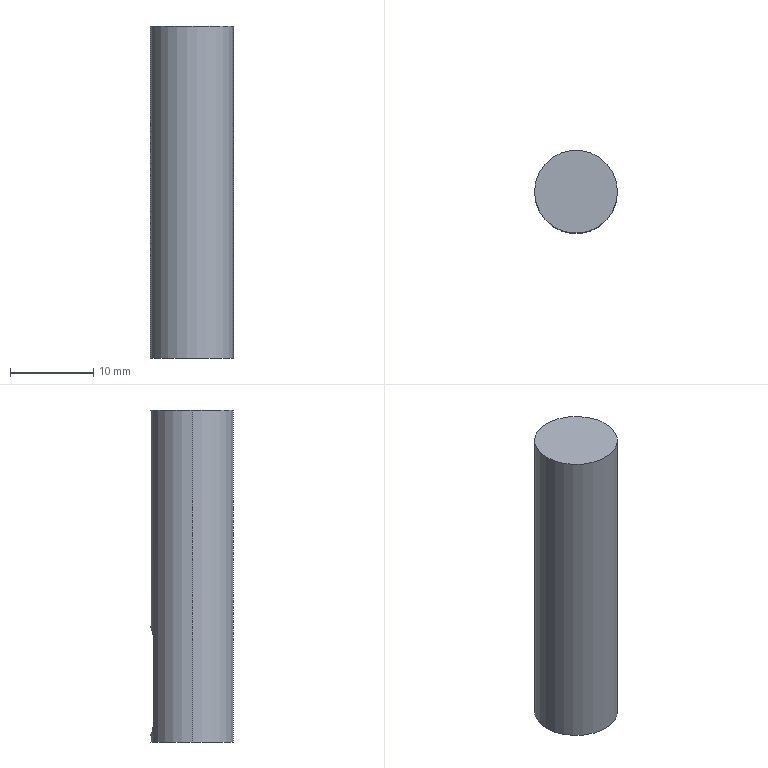Part | SolidWorks | features Extrusion 1, ICE 1 | 1 solid | 10 faces | box 10 x 10 x 40 mm | volume 3009 mm3 | cylinder 5 | plane 5 | commonest cylinder face diameters 3.754 x3 10 x2
STEP:
#1=CARTESIAN_POINT('',(0.,2.,13.877));
#2=VERTEX_POINT('',#1);
#3=CARTESIAN_POINT('',(1.877,2.,12.));
#4=VERTEX_POINT('',#3);
#5=CARTESIAN_POINT('',(0.,2.,12.));
#6=DIRECTION('',(0.,1.,0.));
#7=DIRECTION('',(0.,0.,1.));
#8=AXIS2_PLACEMENT_3D('',#5,#6,#7);
#9=CIRCLE('',#8,1.877);
#10=EDGE_CURVE('',#2,#4,#9,.T.);
#11=ORIENTED_EDGE('',*,*,#10,.F.);
#12=CARTESIAN_POINT('',(0.,5.,13.877));
#13=VERTEX_POINT('',#12);
#14=CARTESIAN_POINT('',(0.,2.,13.877));
#15=DIRECTION('',(0.,1.,0.));
#16=VECTOR('',#15,1000.);
#17=LINE('',#14,#16);
#18=EDGE_CURVE('',#2,#13,#17,.T.);
#19=ORIENTED_EDGE('',*,*,#18,.T.);
#20=CARTESIAN_POINT('',(1.877,4.634,12.));
#21=VERTEX_POINT('',#20);
#22=CARTESIAN_POINT('',(1.877,4.634,12.));
#23=CARTESIAN_POINT('',(1.877,4.634,12.125));
#24=CARTESIAN_POINT('',(1.864,4.639,12.248));
#25=CARTESIAN_POINT('',(1.816,4.659,12.49));
#26=CARTESIAN_POINT('',(1.779,4.673,12.61));
#27=CARTESIAN_POINT('',(1.685,4.708,12.836));
#28=CARTESIAN_POINT('',(1.627,4.728,12.944));
#29=CARTESIAN_POINT('',(1.491,4.773,13.147));
#30=CARTESIAN_POINT('',(1.412,4.797,13.242));
#31=CARTESIAN_POINT('',(1.155,4.868,13.499));
#32=CARTESIAN_POINT('',(0.9475,4.915,13.638));
#33=CARTESIAN_POINT('',(0.609,4.964,13.779));
#34=CARTESIAN_POINT('',(0.4894,4.977,13.816));
#35=CARTESIAN_POINT('',(0.2465,4.995,13.865));
#36=CARTESIAN_POINT('',(0.1238,5.,13.877));
#37=CARTESIAN_POINT('',(0.,5.,13.877));
#38=B_SPLINE_CURVE_WITH_KNOTS('',3,(#22,#23,#24,#25,#26,#27,#28,#29,#30,#31,#32,#33,#34,#35,#36,#37),.UNSPECIFIED.,.F.,.F.,(4,2,2,2,2,2,2,4),(0.,0.0003703,0.0007405,0.001111,0.001481,0.002222,0.002592,0.002962),.UNSPECIFIED.);
#39=EDGE_CURVE('',#21,#13,#38,.T.);
#40=ORIENTED_EDGE('',*,*,#39,.F.);
#41=CARTESIAN_POINT('',(1.877,2.,12.));
#42=DIRECTION('',(0.,1.,0.));
#43=VECTOR('',#42,1000.);
#44=LINE('',#41,#43);
#45=EDGE_CURVE('',#4,#21,#44,.T.);
#46=ORIENTED_EDGE('',*,*,#45,.F.);
#47=EDGE_LOOP('',(#11,#19,#40,#46));
#48=FACE_OUTER_BOUND('',#47,.T.);
#49=CARTESIAN_POINT('',(0.,2.,12.));
#50=DIRECTION('',(0.,1.,0.));
#51=DIRECTION('',(0.,0.,1.));
#52=AXIS2_PLACEMENT_3D('',#49,#50,#51);
#53=CYLINDRICAL_SURFACE('',#52,1.877);
#54=ADVANCED_FACE('',(#48),#53,.F.);
#55=CARTESIAN_POINT('',(-1.877,4.634,12.));
#56=VERTEX_POINT('',#55);
#57=CARTESIAN_POINT('',(-1.877,4.634,2.692));
#58=VERTEX_POINT('',#57);
#59=CARTESIAN_POINT('',(-1.877,4.634,40.));
#60=DIRECTION('',(0.,0.,-1.));
#61=VECTOR('',#60,1000.);
#62=LINE('',#59,#61);
#63=EDGE_CURVE('',#56,#58,#62,.T.);
#64=ORIENTED_EDGE('',*,*,#63,.T.);
#65=CARTESIAN_POINT('',(1.877,4.634,2.692));
#66=VERTEX_POINT('',#65);
#67=CARTESIAN_POINT('',(-1.877,4.634,2.692));
#68=CARTESIAN_POINT('',(-1.877,4.634,2.566));
#69=CARTESIAN_POINT('',(-1.864,4.639,2.444));
#70=CARTESIAN_POINT('',(-1.816,4.659,2.202));
#71=CARTESIAN_POINT('',(-1.779,4.673,2.083));
#72=CARTESIAN_POINT('',(-1.685,4.708,1.856));
#73=CARTESIAN_POINT('',(-1.627,4.728,1.749));
#74=CARTESIAN_POINT('',(-1.491,4.773,1.546));
#75=CARTESIAN_POINT('',(-1.413,4.797,1.45));
#76=CARTESIAN_POINT('',(-1.156,4.868,1.193));
#77=CARTESIAN_POINT('',(-0.9487,4.914,1.054));
#78=CARTESIAN_POINT('',(-0.6107,4.964,0.9127));
#79=CARTESIAN_POINT('',(-0.4912,4.977,0.876));
#80=CARTESIAN_POINT('',(-0.2484,4.995,0.8272));
#81=CARTESIAN_POINT('',(-0.1259,5.,0.8149));
#82=CARTESIAN_POINT('',(0.1215,5.,0.8146));
#83=CARTESIAN_POINT('',(0.2471,4.995,0.827));
#84=CARTESIAN_POINT('',(0.4888,4.978,0.8754));
#85=CARTESIAN_POINT('',(0.6065,4.964,0.9112));
#86=CARTESIAN_POINT('',(0.8353,4.931,1.006));
#87=CARTESIAN_POINT('',(0.9431,4.911,1.064));
#88=CARTESIAN_POINT('',(1.145,4.868,1.2));
#89=CARTESIAN_POINT('',(1.241,4.844,1.278));
#90=CARTESIAN_POINT('',(1.413,4.797,1.45));
#91=CARTESIAN_POINT('',(1.49,4.773,1.544));
#92=CARTESIAN_POINT('',(1.626,4.729,1.746));
#93=CARTESIAN_POINT('',(1.685,4.708,1.856));
#94=CARTESIAN_POINT('',(1.826,4.656,2.194));
#95=CARTESIAN_POINT('',(1.877,4.634,2.441));
#96=CARTESIAN_POINT('',(1.877,4.634,2.692));
#97=B_SPLINE_CURVE_WITH_KNOTS('',3,(#67,#68,#69,#70,#71,#72,#73,#74,#75,#76,#77,#78,#79,#80,#81,#82,#83,#84,#85,#86,#87,#88,#89,#90,#91,#92,#93,#94,#95,#96),.UNSPECIFIED.,.F.,.F.,(4,2,2,2,2,2,2,2,2,2,2,2,2,2,4),(0.,0.00037,0.00074,0.00111,0.00148,0.00222,0.00259,0.00296,0.00333,0.0037,0.00407,0.00444,0.00481,0.00518,0.00592),.UNSPECIFIED.);
#98=EDGE_CURVE('',#58,#66,#97,.T.);
#99=ORIENTED_EDGE('',*,*,#98,.T.);
#100=CARTESIAN_POINT('',(1.877,4.634,40.));
#101=DIRECTION('',(0.,0.,1.));
#102=VECTOR('',#101,1000.);
#103=LINE('',#100,#102);
#104=EDGE_CURVE('',#66,#21,#103,.T.);
#105=ORIENTED_EDGE('',*,*,#104,.T.);
#106=ORIENTED_EDGE('',*,*,#39,.T.);
#107=CARTESIAN_POINT('',(0.,5.,13.877));
#108=CARTESIAN_POINT('',(-0.1236,5.,13.877));
#109=CARTESIAN_POINT('',(-0.2491,4.995,13.864));
#110=CARTESIAN_POINT('',(-0.4906,4.977,13.816));
#111=CARTESIAN_POINT('',(-0.6081,4.964,13.78));
#112=CARTESIAN_POINT('',(-0.8367,4.931,13.685));
#113=CARTESIAN_POINT('',(-0.9443,4.911,13.626));
#114=CARTESIAN_POINT('',(-1.146,4.868,13.491));
#115=CARTESIAN_POINT('',(-1.242,4.844,13.413));
#116=CARTESIAN_POINT('',(-1.414,4.797,13.241));
#117=CARTESIAN_POINT('',(-1.491,4.773,13.147));
#118=CARTESIAN_POINT('',(-1.626,4.729,12.945));
#119=CARTESIAN_POINT('',(-1.685,4.708,12.835));
#120=CARTESIAN_POINT('',(-1.826,4.656,12.498));
#121=CARTESIAN_POINT('',(-1.877,4.634,12.25));
#122=CARTESIAN_POINT('',(-1.877,4.634,12.));
#123=B_SPLINE_CURVE_WITH_KNOTS('',3,(#107,#108,#109,#110,#111,#112,#113,#114,#115,#116,#117,#118,#119,#120,#121,#122),.UNSPECIFIED.,.F.,.F.,(4,2,2,2,2,2,2,4),(0.002962,0.003332,0.003702,0.004071,0.004441,0.004811,0.00518,0.00592),.UNSPECIFIED.);
#124=EDGE_CURVE('',#13,#56,#123,.T.);
#125=ORIENTED_EDGE('',*,*,#124,.T.);
#126=EDGE_LOOP('',(#64,#99,#105,#106,#125));
#127=FACE_BOUND('',#126,.T.);
#128=CARTESIAN_POINT('',(5.,0.,40.));
#129=VERTEX_POINT('',#128);
#130=CARTESIAN_POINT('',(-5.,0.,40.));
#131=VERTEX_POINT('',#130);
#132=CARTESIAN_POINT('',(0.,0.,40.));
#133=DIRECTION('',(0.,0.,1.));
#134=DIRECTION('',(1.,0.,0.));
#135=AXIS2_PLACEMENT_3D('',#132,#133,#134);
#136=CIRCLE('',#135,5.);
#137=EDGE_CURVE('',#129,#131,#136,.T.);
#138=ORIENTED_EDGE('',*,*,#137,.F.);
#139=CARTESIAN_POINT('',(5.,0.,0.));
#140=VERTEX_POINT('',#139);
#141=CARTESIAN_POINT('',(5.,0.,40.));
#142=DIRECTION('',(0.,0.,-1.));
#143=VECTOR('',#142,1000.);
#144=LINE('',#141,#143);
#145=EDGE_CURVE('',#129,#140,#144,.T.);
#146=ORIENTED_EDGE('',*,*,#145,.T.);
#147=CARTESIAN_POINT('',(-5.,0.,0.));
#148=VERTEX_POINT('',#147);
#149=CARTESIAN_POINT('',(0.,0.,0.));
#150=DIRECTION('',(0.,0.,1.));
#151=DIRECTION('',(1.,0.,0.));
#152=AXIS2_PLACEMENT_3D('',#149,#150,#151);
#153=CIRCLE('',#152,5.);
#154=EDGE_CURVE('',#140,#148,#153,.T.);
#155=ORIENTED_EDGE('',*,*,#154,.T.);
#156=CARTESIAN_POINT('',(-5.,0.,40.));
#157=DIRECTION('',(0.,0.,-1.));
#158=VECTOR('',#157,1000.);
#159=LINE('',#156,#158);
#160=EDGE_CURVE('',#131,#148,#159,.T.);
#161=ORIENTED_EDGE('',*,*,#160,.F.);
#162=EDGE_LOOP('',(#138,#146,#155,#161));
#163=FACE_OUTER_BOUND('',#162,.T.);
#164=CARTESIAN_POINT('',(0.,0.,40.));
#165=DIRECTION('',(0.,0.,-1.));
#166=DIRECTION('',(-1.,0.,0.));
#167=AXIS2_PLACEMENT_3D('',#164,#165,#166);
#168=CYLINDRICAL_SURFACE('',#167,5.);
#169=ADVANCED_FACE('',(#127,#163),#168,.T.);
#170=ORIENTED_EDGE('',*,*,#145,.F.);
#171=CARTESIAN_POINT('',(0.,0.,40.));
#172=DIRECTION('',(0.,0.,1.));
#173=DIRECTION('',(1.,0.,0.));
#174=AXIS2_PLACEMENT_3D('',#171,#172,#173);
#175=CIRCLE('',#174,5.);
#176=EDGE_CURVE('',#131,#129,#175,.T.);
#177=ORIENTED_EDGE('',*,*,#176,.F.);
#178=ORIENTED_EDGE('',*,*,#160,.T.);
#179=CARTESIAN_POINT('',(0.,0.,0.));
#180=DIRECTION('',(0.,0.,1.));
#181=DIRECTION('',(1.,0.,0.));
#182=AXIS2_PLACEMENT_3D('',#179,#180,#181);
#183=CIRCLE('',#182,5.);
#184=EDGE_CURVE('',#148,#140,#183,.T.);
#185=ORIENTED_EDGE('',*,*,#184,.T.);
#186=EDGE_LOOP('',(#170,#177,#178,#185));
#187=FACE_OUTER_BOUND('',#186,.T.);
#188=CARTESIAN_POINT('',(0.,0.,40.));
#189=DIRECTION('',(0.,0.,-1.));
#190=DIRECTION('',(-1.,0.,0.));
#191=AXIS2_PLACEMENT_3D('',#188,#189,#190);
#192=CYLINDRICAL_SURFACE('',#191,5.);
#193=ADVANCED_FACE('',(#187),#192,.T.);
#194=ORIENTED_EDGE('',*,*,#176,.T.);
#195=ORIENTED_EDGE('',*,*,#137,.T.);
#196=EDGE_LOOP('',(#194,#195));
#197=FACE_OUTER_BOUND('',#196,.T.);
#198=CARTESIAN_POINT('',(0.,0.,40.));
#199=DIRECTION('',(0.,0.,1.));
#200=DIRECTION('',(1.,0.,0.));
#201=AXIS2_PLACEMENT_3D('',#198,#199,#200);
#202=PLANE('',#201);
#203=ADVANCED_FACE('',(#197),#202,.T.);
#204=ORIENTED_EDGE('',*,*,#184,.F.);
#205=ORIENTED_EDGE('',*,*,#154,.F.);
#206=EDGE_LOOP('',(#204,#205));
#207=FACE_OUTER_BOUND('',#206,.T.);
#208=CARTESIAN_POINT('',(0.,0.,0.));
#209=DIRECTION('',(0.,0.,1.));
#210=DIRECTION('',(1.,0.,0.));
#211=AXIS2_PLACEMENT_3D('',#208,#209,#210);
#212=PLANE('',#211);
#213=ADVANCED_FACE('',(#207),#212,.F.);
#214=ORIENTED_EDGE('',*,*,#18,.F.);
#215=CARTESIAN_POINT('',(-1.877,2.,12.));
#216=VERTEX_POINT('',#215);
#217=CARTESIAN_POINT('',(0.,2.,12.));
#218=DIRECTION('',(0.,1.,0.));
#219=DIRECTION('',(0.,0.,1.));
#220=AXIS2_PLACEMENT_3D('',#217,#218,#219);
#221=CIRCLE('',#220,1.877);
#222=EDGE_CURVE('',#216,#2,#221,.T.);
#223=ORIENTED_EDGE('',*,*,#222,.F.);
#224=CARTESIAN_POINT('',(-1.877,2.,12.));
#225=DIRECTION('',(0.,1.,0.));
#226=VECTOR('',#225,1000.);
#227=LINE('',#224,#226);
#228=EDGE_CURVE('',#216,#56,#227,.T.);
#229=ORIENTED_EDGE('',*,*,#228,.T.);
#230=ORIENTED_EDGE('',*,*,#124,.F.);
#231=EDGE_LOOP('',(#214,#223,#229,#230));
#232=FACE_OUTER_BOUND('',#231,.T.);
#233=CARTESIAN_POINT('',(0.,2.,12.));
#234=DIRECTION('',(0.,1.,0.));
#235=DIRECTION('',(0.,0.,1.));
#236=AXIS2_PLACEMENT_3D('',#233,#234,#235);
#237=CYLINDRICAL_SURFACE('',#236,1.877);
#238=ADVANCED_FACE('',(#232),#237,.F.);
#239=ORIENTED_EDGE('',*,*,#228,.F.);
#240=CARTESIAN_POINT('',(-1.877,2.,2.692));
#241=VERTEX_POINT('',#240);
#242=CARTESIAN_POINT('',(-1.877,2.,12.));
#243=DIRECTION('',(0.,0.,1.));
#244=VECTOR('',#243,1000.);
#245=LINE('',#242,#244);
#246=EDGE_CURVE('',#241,#216,#245,.T.);
#247=ORIENTED_EDGE('',*,*,#246,.F.);
#248=CARTESIAN_POINT('',(-1.877,2.,2.692));
#249=DIRECTION('',(0.,1.,0.));
#250=VECTOR('',#249,1000.);
#251=LINE('',#248,#250);
#252=EDGE_CURVE('',#241,#58,#251,.T.);
#253=ORIENTED_EDGE('',*,*,#252,.T.);
#254=ORIENTED_EDGE('',*,*,#63,.F.);
#255=EDGE_LOOP('',(#239,#247,#253,#254));
#256=FACE_OUTER_BOUND('',#255,.T.);
#257=CARTESIAN_POINT('',(-1.877,2.,12.));
#258=DIRECTION('',(-1.,0.,0.));
#259=DIRECTION('',(0.,0.,1.));
#260=AXIS2_PLACEMENT_3D('',#257,#258,#259);
#261=PLANE('',#260);
#262=ADVANCED_FACE('',(#256),#261,.F.);
#263=ORIENTED_EDGE('',*,*,#252,.F.);
#264=CARTESIAN_POINT('',(1.877,2.,2.692));
#265=VERTEX_POINT('',#264);
#266=CARTESIAN_POINT('',(0.,2.,2.692));
#267=DIRECTION('',(0.,1.,0.));
#268=DIRECTION('',(0.,0.,1.));
#269=AXIS2_PLACEMENT_3D('',#266,#267,#268);
#270=CIRCLE('',#269,1.877);
#271=EDGE_CURVE('',#265,#241,#270,.T.);
#272=ORIENTED_EDGE('',*,*,#271,.F.);
#273=CARTESIAN_POINT('',(1.877,2.,2.692));
#274=DIRECTION('',(0.,1.,0.));
#275=VECTOR('',#274,1000.);
#276=LINE('',#273,#275);
#277=EDGE_CURVE('',#265,#66,#276,.T.);
#278=ORIENTED_EDGE('',*,*,#277,.T.);
#279=ORIENTED_EDGE('',*,*,#98,.F.);
#280=EDGE_LOOP('',(#263,#272,#278,#279));
#281=FACE_OUTER_BOUND('',#280,.T.);
#282=CARTESIAN_POINT('',(0.,2.,2.692));
#283=DIRECTION('',(0.,1.,0.));
#284=DIRECTION('',(0.,0.,1.));
#285=AXIS2_PLACEMENT_3D('',#282,#283,#284);
#286=CYLINDRICAL_SURFACE('',#285,1.877);
#287=ADVANCED_FACE('',(#281),#286,.F.);
#288=ORIENTED_EDGE('',*,*,#277,.F.);
#289=CARTESIAN_POINT('',(1.877,2.,12.));
#290=DIRECTION('',(0.,0.,-1.));
#291=VECTOR('',#290,1000.);
#292=LINE('',#289,#291);
#293=EDGE_CURVE('',#4,#265,#292,.T.);
#294=ORIENTED_EDGE('',*,*,#293,.F.);
#295=ORIENTED_EDGE('',*,*,#45,.T.);
#296=ORIENTED_EDGE('',*,*,#104,.F.);
#297=EDGE_LOOP('',(#288,#294,#295,#296));
#298=FACE_OUTER_BOUND('',#297,.T.);
#299=CARTESIAN_POINT('',(1.877,2.,12.));
#300=DIRECTION('',(1.,0.,0.));
#301=DIRECTION('',(0.,0.,-1.));
#302=AXIS2_PLACEMENT_3D('',#299,#300,#301);
#303=PLANE('',#302);
#304=ADVANCED_FACE('',(#298),#303,.F.);
#305=ORIENTED_EDGE('',*,*,#222,.T.);
#306=ORIENTED_EDGE('',*,*,#10,.T.);
#307=ORIENTED_EDGE('',*,*,#293,.T.);
#308=ORIENTED_EDGE('',*,*,#271,.T.);
#309=ORIENTED_EDGE('',*,*,#246,.T.);
#310=EDGE_LOOP('',(#305,#306,#307,#308,#309));
#311=FACE_OUTER_BOUND('',#310,.T.);
#312=CARTESIAN_POINT('',(0.,2.,12.));
#313=DIRECTION('',(0.,1.,0.));
#314=DIRECTION('',(0.,0.,1.));
#315=AXIS2_PLACEMENT_3D('',#312,#313,#314);
#316=PLANE('',#315);
#317=ADVANCED_FACE('',(#311),#316,.T.);
#318=CLOSED_SHELL('',(#54,#169,#193,#203,#213,#238,#262,#287,#304,#317));
#319=MANIFOLD_SOLID_BREP('',#318);
#320=CARTESIAN_POINT('',(0.,0.,0.));
#321=DIRECTION('',(0.,0.,1.));
#322=DIRECTION('',(1.,0.,0.));
#323=AXIS2_PLACEMENT_3D('',#320,#321,#322);
#324=(LENGTH_UNIT()NAMED_UNIT(*)SI_UNIT(.MILLI.,.METRE.));
#325=UNCERTAINTY_MEASURE_WITH_UNIT(LENGTH_MEASURE(0.00001),#324,'','');
#326=(NAMED_UNIT(*)PLANE_ANGLE_UNIT()SI_UNIT($,.RADIAN.));
#327=(NAMED_UNIT(*)SI_UNIT($,.STERADIAN.)SOLID_ANGLE_UNIT());
#328=(GEOMETRIC_REPRESENTATION_CONTEXT(3)GLOBAL_UNCERTAINTY_ASSIGNED_CONTEXT((#325))GLOBAL_UNIT_ASSIGNED_CONTEXT((#324,#326,#327))REPRESENTATION_CONTEXT('',''));
#329=ADVANCED_BREP_SHAPE_REPRESENTATION('',(#319,#323),#328);